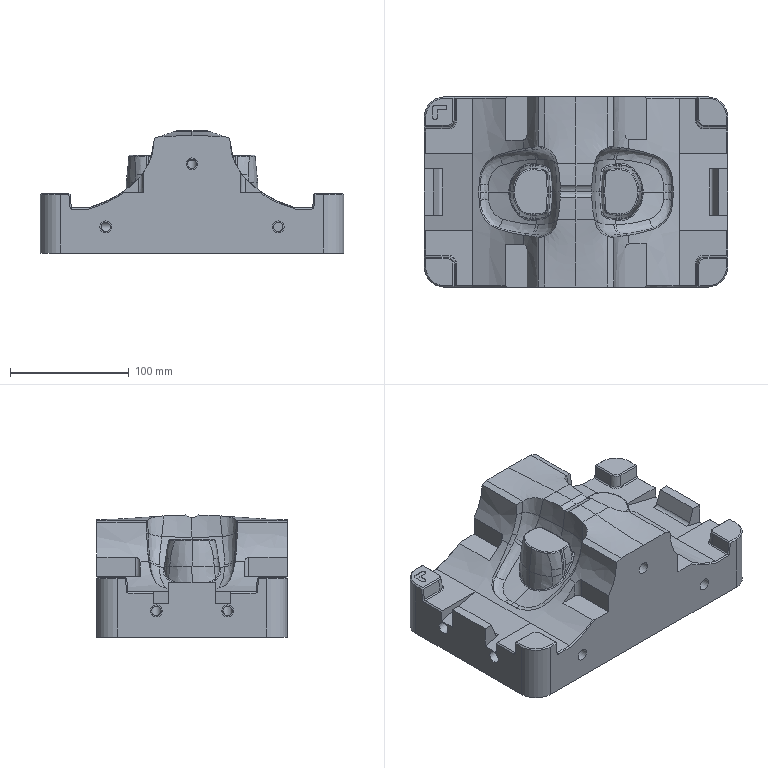Part | 1 solid | 406 faces | box 255 x 160 x 102.619 mm | volume 2315331 mm3 | spline 172 | plane 120 | cylinder 92 | cone 18 | sphere 4 | commonest cylinder face diameters 8 x32 2 x16 10 x9 2.014 x4 12 x4 34 x4